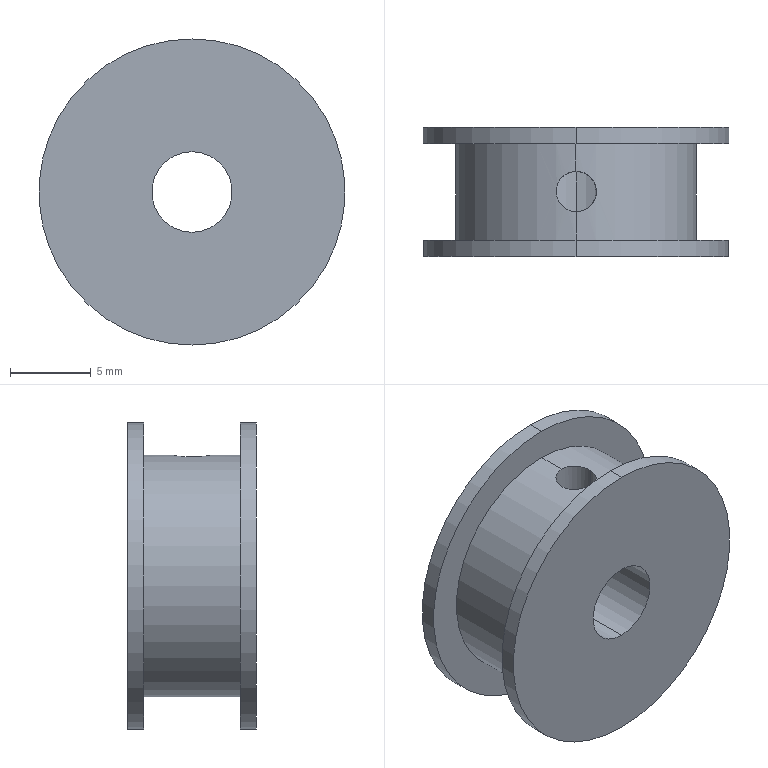Part | SolidWorks | features 3DProfileFeature 1, HoleWzd 1, Revolution 1 | 1 solid | 14 faces | box 19 x 8 x 19 mm | volume 1445 mm3 | cylinder 10 | plane 4 | commonest cylinder face diameters 19 x4 2.5 x2 5 x2 15 x2
STEP:
#1=CARTESIAN_POINT('',(-1.244,5.135,2.168));
#2=VERTEX_POINT('',#1);
#3=CARTESIAN_POINT('',(0.,3.885,2.5));
#4=VERTEX_POINT('',#3);
#5=CARTESIAN_POINT('',(-1.244,5.135,2.168));
#6=CARTESIAN_POINT('',(-1.244,5.053,2.168));
#7=CARTESIAN_POINT('',(-1.236,4.969,2.173));
#8=CARTESIAN_POINT('',(-1.203,4.808,2.191));
#9=CARTESIAN_POINT('',(-1.179,4.73,2.205));
#10=CARTESIAN_POINT('',(-1.085,4.503,2.253));
#11=CARTESIAN_POINT('',(-0.9937,4.368,2.297));
#12=CARTESIAN_POINT('',(-0.8237,4.197,2.361));
#13=CARTESIAN_POINT('',(-0.7622,4.146,2.382));
#14=CARTESIAN_POINT('',(-0.6291,4.056,2.421));
#15=CARTESIAN_POINT('',(-0.5566,4.016,2.438));
#16=CARTESIAN_POINT('',(-0.3321,3.921,2.483));
#17=CARTESIAN_POINT('',(-0.1673,3.886,2.5));
#18=CARTESIAN_POINT('',(0.,3.885,2.5));
#19=B_SPLINE_CURVE_WITH_KNOTS('',3,(#5,#6,#7,#8,#9,#10,#11,#12,#13,#14,#15,#16,#17,#18),.UNSPECIFIED.,.F.,.F.,(4,2,2,2,2,2,4),(0.005969,0.006216,0.006463,0.006957,0.007204,0.007451,0.007946),.UNSPECIFIED.);
#20=EDGE_CURVE('',#2,#4,#19,.T.);
#21=ORIENTED_EDGE('',*,*,#20,.F.);
#22=CARTESIAN_POINT('',(-1.231,5.135,7.398));
#23=VERTEX_POINT('',#22);
#24=CARTESIAN_POINT('',(-1.23,5.135,7.503));
#25=DIRECTION('',(0.002602,0.,1.));
#26=VECTOR('',#25,1000.);
#27=LINE('',#24,#26);
#28=EDGE_CURVE('',#2,#23,#27,.T.);
#29=ORIENTED_EDGE('',*,*,#28,.T.);
#30=CARTESIAN_POINT('',(0.,3.886,7.5));
#31=VERTEX_POINT('',#30);
#32=CARTESIAN_POINT('',(0.,3.886,7.5));
#33=CARTESIAN_POINT('',(-0.1639,3.888,7.5));
#34=CARTESIAN_POINT('',(-0.3241,3.923,7.494));
#35=CARTESIAN_POINT('',(-0.6224,4.051,7.476));
#36=CARTESIAN_POINT('',(-0.7586,4.144,7.462));
#37=CARTESIAN_POINT('',(-0.9848,4.374,7.436));
#38=CARTESIAN_POINT('',(-1.076,4.512,7.423));
#39=CARTESIAN_POINT('',(-1.198,4.811,7.404));
#40=CARTESIAN_POINT('',(-1.231,4.974,7.398));
#41=CARTESIAN_POINT('',(-1.231,5.135,7.398));
#42=B_SPLINE_CURVE_WITH_KNOTS('',3,(#32,#33,#34,#35,#36,#37,#38,#39,#40,#41),.UNSPECIFIED.,.F.,.F.,(4,2,2,2,4),(0.,0.0004846,0.0009692,0.001454,0.001938),.UNSPECIFIED.);
#43=EDGE_CURVE('',#31,#23,#42,.T.);
#44=ORIENTED_EDGE('',*,*,#43,.F.);
#45=CARTESIAN_POINT('',(1.269,5.135,7.392));
#46=VERTEX_POINT('',#45);
#47=CARTESIAN_POINT('',(1.269,5.135,7.392));
#48=CARTESIAN_POINT('',(1.269,4.969,7.392));
#49=CARTESIAN_POINT('',(1.236,4.805,7.398));
#50=CARTESIAN_POINT('',(1.108,4.5,7.418));
#51=CARTESIAN_POINT('',(1.014,4.36,7.432));
#52=CARTESIAN_POINT('',(0.7796,4.13,7.46));
#53=CARTESIAN_POINT('',(0.6382,4.037,7.474));
#54=CARTESIAN_POINT('',(0.3334,3.914,7.494));
#55=CARTESIAN_POINT('',(0.167,3.883,7.5));
#56=CARTESIAN_POINT('',(0.,3.886,7.5));
#57=B_SPLINE_CURVE_WITH_KNOTS('',3,(#47,#48,#49,#50,#51,#52,#53,#54,#55,#56),.UNSPECIFIED.,.F.,.F.,(4,2,2,2,4),(0.005853,0.006347,0.006841,0.007335,0.007829),.UNSPECIFIED.);
#58=EDGE_CURVE('',#46,#31,#57,.T.);
#59=ORIENTED_EDGE('',*,*,#58,.F.);
#60=CARTESIAN_POINT('',(1.256,5.135,2.162));
#61=VERTEX_POINT('',#60);
#62=CARTESIAN_POINT('',(1.27,5.135,7.497));
#63=DIRECTION('',(0.002602,0.,1.));
#64=VECTOR('',#63,1000.);
#65=LINE('',#62,#64);
#66=EDGE_CURVE('',#61,#46,#65,.T.);
#67=ORIENTED_EDGE('',*,*,#66,.F.);
#68=CARTESIAN_POINT('',(0.,3.885,2.5));
#69=CARTESIAN_POINT('',(0.08444,3.885,2.5));
#70=CARTESIAN_POINT('',(0.1673,3.893,2.496));
#71=CARTESIAN_POINT('',(0.3298,3.925,2.479));
#72=CARTESIAN_POINT('',(0.4104,3.95,2.467));
#73=CARTESIAN_POINT('',(0.638,4.044,2.422));
#74=CARTESIAN_POINT('',(0.7754,4.137,2.38));
#75=CARTESIAN_POINT('',(1.003,4.364,2.293));
#76=CARTESIAN_POINT('',(1.095,4.501,2.248));
#77=CARTESIAN_POINT('',(1.19,4.727,2.199));
#78=CARTESIAN_POINT('',(1.215,4.807,2.185));
#79=CARTESIAN_POINT('',(1.247,4.97,2.167));
#80=CARTESIAN_POINT('',(1.256,5.052,2.162));
#81=CARTESIAN_POINT('',(1.256,5.135,2.162));
#82=B_SPLINE_CURVE_WITH_KNOTS('',3,(#68,#69,#70,#71,#72,#73,#74,#75,#76,#77,#78,#79,#80,#81),.UNSPECIFIED.,.F.,.F.,(4,2,2,2,2,2,4),(0.,0.0002495,0.000499,0.0009979,0.001497,0.001746,0.001996),.UNSPECIFIED.);
#83=EDGE_CURVE('',#4,#61,#82,.T.);
#84=ORIENTED_EDGE('',*,*,#83,.F.);
#85=EDGE_LOOP('',(#21,#29,#44,#59,#67,#84));
#86=FACE_OUTER_BOUND('',#85,.T.);
#87=CARTESIAN_POINT('',(0.01951,5.135,7.5));
#88=DIRECTION('',(0.002602,0.,1.));
#89=DIRECTION('',(1.,0.,-0.002602));
#90=AXIS2_PLACEMENT_3D('',#87,#88,#89);
#91=CYLINDRICAL_SURFACE('',#90,1.25);
#92=ADVANCED_FACE('',(#86),#91,.F.);
#93=CARTESIAN_POINT('',(0.,1.117,-2.5));
#94=VERTEX_POINT('',#93);
#95=CARTESIAN_POINT('',(0.,1.117,2.5));
#96=VERTEX_POINT('',#95);
#97=CARTESIAN_POINT('',(0.,1.117,0.));
#98=DIRECTION('',(0.,1.,0.));
#99=DIRECTION('',(0.,0.,1.));
#100=AXIS2_PLACEMENT_3D('',#97,#98,#99);
#101=CIRCLE('',#100,2.5);
#102=EDGE_CURVE('',#94,#96,#101,.T.);
#103=ORIENTED_EDGE('',*,*,#102,.F.);
#104=CARTESIAN_POINT('',(0.,9.117,-2.5));
#105=VERTEX_POINT('',#104);
#106=CARTESIAN_POINT('',(0.,18.914,-2.5));
#107=DIRECTION('',(0.,1.,0.));
#108=VECTOR('',#107,1000.);
#109=LINE('',#106,#108);
#110=EDGE_CURVE('',#94,#105,#109,.T.);
#111=ORIENTED_EDGE('',*,*,#110,.T.);
#112=CARTESIAN_POINT('',(0.,9.117,2.5));
#113=VERTEX_POINT('',#112);
#114=CARTESIAN_POINT('',(0.,9.117,0.));
#115=DIRECTION('',(0.,1.,0.));
#116=DIRECTION('',(0.,0.,1.));
#117=AXIS2_PLACEMENT_3D('',#114,#115,#116);
#118=CIRCLE('',#117,2.5);
#119=EDGE_CURVE('',#105,#113,#118,.T.);
#120=ORIENTED_EDGE('',*,*,#119,.T.);
#121=CARTESIAN_POINT('',(0.,6.385,2.5));
#122=VERTEX_POINT('',#121);
#123=CARTESIAN_POINT('',(0.,18.914,2.5));
#124=DIRECTION('',(0.,1.,0.));
#125=VECTOR('',#124,1000.);
#126=LINE('',#123,#125);
#127=EDGE_CURVE('',#122,#113,#126,.T.);
#128=ORIENTED_EDGE('',*,*,#127,.F.);
#129=CARTESIAN_POINT('',(0.,6.385,2.5));
#130=CARTESIAN_POINT('',(-0.08271,6.385,2.5));
#131=CARTESIAN_POINT('',(-0.1668,6.376,2.496));
#132=CARTESIAN_POINT('',(-0.3281,6.343,2.48));
#133=CARTESIAN_POINT('',(-0.4065,6.318,2.468));
#134=CARTESIAN_POINT('',(-0.634,6.222,2.423));
#135=CARTESIAN_POINT('',(-0.7689,6.129,2.382));
#136=CARTESIAN_POINT('',(-0.9946,5.902,2.297));
#137=CARTESIAN_POINT('',(-1.086,5.765,2.253));
#138=CARTESIAN_POINT('',(-1.21,5.467,2.189));
#139=CARTESIAN_POINT('',(-1.244,5.3,2.168));
#140=CARTESIAN_POINT('',(-1.244,5.135,2.168));
#141=B_SPLINE_CURVE_WITH_KNOTS('',3,(#129,#130,#131,#132,#133,#134,#135,#136,#137,#138,#139,#140),.UNSPECIFIED.,.F.,.F.,(4,2,2,2,2,4),(0.003989,0.004237,0.004484,0.004979,0.005474,0.005969),.UNSPECIFIED.);
#142=EDGE_CURVE('',#122,#2,#141,.T.);
#143=ORIENTED_EDGE('',*,*,#142,.T.);
#144=ORIENTED_EDGE('',*,*,#20,.T.);
#145=CARTESIAN_POINT('',(0.,18.914,2.5));
#146=DIRECTION('',(0.,1.,0.));
#147=VECTOR('',#146,1000.);
#148=LINE('',#145,#147);
#149=EDGE_CURVE('',#96,#4,#148,.T.);
#150=ORIENTED_EDGE('',*,*,#149,.F.);
#151=EDGE_LOOP('',(#103,#111,#120,#128,#143,#144,#150));
#152=FACE_OUTER_BOUND('',#151,.T.);
#153=CARTESIAN_POINT('',(0.,18.914,0.));
#154=DIRECTION('',(0.,1.,0.));
#155=DIRECTION('',(0.,0.,1.));
#156=AXIS2_PLACEMENT_3D('',#153,#154,#155);
#157=CYLINDRICAL_SURFACE('',#156,2.5);
#158=ADVANCED_FACE('',(#152),#157,.F.);
#159=CARTESIAN_POINT('',(0.,1.117,9.5));
#160=VERTEX_POINT('',#159);
#161=CARTESIAN_POINT('',(0.,1.117,-9.5));
#162=VERTEX_POINT('',#161);
#163=CARTESIAN_POINT('',(0.,1.117,0.));
#164=DIRECTION('',(0.,1.,0.));
#165=DIRECTION('',(0.,0.,1.));
#166=AXIS2_PLACEMENT_3D('',#163,#164,#165);
#167=CIRCLE('',#166,9.5);
#168=EDGE_CURVE('',#160,#162,#167,.T.);
#169=ORIENTED_EDGE('',*,*,#168,.T.);
#170=CARTESIAN_POINT('',(0.,2.117,-9.5));
#171=VERTEX_POINT('',#170);
#172=CARTESIAN_POINT('',(0.,18.914,-9.5));
#173=DIRECTION('',(0.,1.,0.));
#174=VECTOR('',#173,1000.);
#175=LINE('',#172,#174);
#176=EDGE_CURVE('',#162,#171,#175,.T.);
#177=ORIENTED_EDGE('',*,*,#176,.T.);
#178=CARTESIAN_POINT('',(0.,2.117,9.5));
#179=VERTEX_POINT('',#178);
#180=CARTESIAN_POINT('',(0.,2.117,0.));
#181=DIRECTION('',(0.,1.,0.));
#182=DIRECTION('',(0.,0.,1.));
#183=AXIS2_PLACEMENT_3D('',#180,#181,#182);
#184=CIRCLE('',#183,9.5);
#185=EDGE_CURVE('',#179,#171,#184,.T.);
#186=ORIENTED_EDGE('',*,*,#185,.F.);
#187=CARTESIAN_POINT('',(0.,18.914,9.5));
#188=DIRECTION('',(0.,1.,0.));
#189=VECTOR('',#188,1000.);
#190=LINE('',#187,#189);
#191=EDGE_CURVE('',#160,#179,#190,.T.);
#192=ORIENTED_EDGE('',*,*,#191,.F.);
#193=EDGE_LOOP('',(#169,#177,#186,#192));
#194=FACE_OUTER_BOUND('',#193,.T.);
#195=CARTESIAN_POINT('',(0.,18.914,0.));
#196=DIRECTION('',(0.,1.,0.));
#197=DIRECTION('',(0.,0.,1.));
#198=AXIS2_PLACEMENT_3D('',#195,#196,#197);
#199=CYLINDRICAL_SURFACE('',#198,9.5);
#200=ADVANCED_FACE('',(#194),#199,.T.);
#201=CARTESIAN_POINT('',(0.,2.117,7.5));
#202=VERTEX_POINT('',#201);
#203=CARTESIAN_POINT('',(0.,2.117,-7.5));
#204=VERTEX_POINT('',#203);
#205=CARTESIAN_POINT('',(0.,2.117,0.));
#206=DIRECTION('',(0.,1.,0.));
#207=DIRECTION('',(0.,0.,1.));
#208=AXIS2_PLACEMENT_3D('',#205,#206,#207);
#209=CIRCLE('',#208,7.5);
#210=EDGE_CURVE('',#202,#204,#209,.T.);
#211=ORIENTED_EDGE('',*,*,#210,.T.);
#212=CARTESIAN_POINT('',(0.,8.117,-7.5));
#213=VERTEX_POINT('',#212);
#214=CARTESIAN_POINT('',(0.,18.914,-7.5));
#215=DIRECTION('',(0.,1.,0.));
#216=VECTOR('',#215,1000.);
#217=LINE('',#214,#216);
#218=EDGE_CURVE('',#204,#213,#217,.T.);
#219=ORIENTED_EDGE('',*,*,#218,.T.);
#220=CARTESIAN_POINT('',(0.,8.117,7.5));
#221=VERTEX_POINT('',#220);
#222=CARTESIAN_POINT('',(0.,8.117,0.));
#223=DIRECTION('',(0.,1.,0.));
#224=DIRECTION('',(0.,0.,1.));
#225=AXIS2_PLACEMENT_3D('',#222,#223,#224);
#226=CIRCLE('',#225,7.5);
#227=EDGE_CURVE('',#221,#213,#226,.T.);
#228=ORIENTED_EDGE('',*,*,#227,.F.);
#229=CARTESIAN_POINT('',(0.,6.385,7.5));
#230=VERTEX_POINT('',#229);
#231=CARTESIAN_POINT('',(0.,18.914,7.5));
#232=DIRECTION('',(0.,1.,0.));
#233=VECTOR('',#232,1000.);
#234=LINE('',#231,#233);
#235=EDGE_CURVE('',#230,#221,#234,.T.);
#236=ORIENTED_EDGE('',*,*,#235,.F.);
#237=CARTESIAN_POINT('',(0.,6.385,7.5));
#238=CARTESIAN_POINT('',(0.1653,6.388,7.5));
#239=CARTESIAN_POINT('',(0.3319,6.357,7.494));
#240=CARTESIAN_POINT('',(0.6374,6.234,7.474));
#241=CARTESIAN_POINT('',(0.779,6.142,7.46));
#242=CARTESIAN_POINT('',(1.013,5.911,7.432));
#243=CARTESIAN_POINT('',(1.108,5.772,7.418));
#244=CARTESIAN_POINT('',(1.236,5.467,7.398));
#245=CARTESIAN_POINT('',(1.269,5.303,7.392));
#246=CARTESIAN_POINT('',(1.269,5.135,7.392));
#247=B_SPLINE_CURVE_WITH_KNOTS('',3,(#237,#238,#239,#240,#241,#242,#243,#244,#245,#246),.UNSPECIFIED.,.F.,.F.,(4,2,2,2,4),(0.003876,0.00437,0.004865,0.005359,0.005853),.UNSPECIFIED.);
#248=EDGE_CURVE('',#230,#46,#247,.T.);
#249=ORIENTED_EDGE('',*,*,#248,.T.);
#250=ORIENTED_EDGE('',*,*,#58,.T.);
#251=CARTESIAN_POINT('',(0.,18.914,7.5));
#252=DIRECTION('',(0.,1.,0.));
#253=VECTOR('',#252,1000.);
#254=LINE('',#251,#253);
#255=EDGE_CURVE('',#202,#31,#254,.T.);
#256=ORIENTED_EDGE('',*,*,#255,.F.);
#257=EDGE_LOOP('',(#211,#219,#228,#236,#249,#250,#256));
#258=FACE_OUTER_BOUND('',#257,.T.);
#259=CARTESIAN_POINT('',(0.,18.914,0.));
#260=DIRECTION('',(0.,1.,0.));
#261=DIRECTION('',(0.,0.,1.));
#262=AXIS2_PLACEMENT_3D('',#259,#260,#261);
#263=CYLINDRICAL_SURFACE('',#262,7.5);
#264=ADVANCED_FACE('',(#258),#263,.T.);
#265=CARTESIAN_POINT('',(0.,8.117,9.5));
#266=VERTEX_POINT('',#265);
#267=CARTESIAN_POINT('',(0.,8.117,-9.5));
#268=VERTEX_POINT('',#267);
#269=CARTESIAN_POINT('',(0.,8.117,0.));
#270=DIRECTION('',(0.,1.,0.));
#271=DIRECTION('',(0.,0.,1.));
#272=AXIS2_PLACEMENT_3D('',#269,#270,#271);
#273=CIRCLE('',#272,9.5);
#274=EDGE_CURVE('',#266,#268,#273,.T.);
#275=ORIENTED_EDGE('',*,*,#274,.T.);
#276=CARTESIAN_POINT('',(0.,9.117,-9.5));
#277=VERTEX_POINT('',#276);
#278=CARTESIAN_POINT('',(0.,18.914,-9.5));
#279=DIRECTION('',(0.,1.,0.));
#280=VECTOR('',#279,1000.);
#281=LINE('',#278,#280);
#282=EDGE_CURVE('',#268,#277,#281,.T.);
#283=ORIENTED_EDGE('',*,*,#282,.T.);
#284=CARTESIAN_POINT('',(0.,9.117,9.5));
#285=VERTEX_POINT('',#284);
#286=CARTESIAN_POINT('',(0.,9.117,0.));
#287=DIRECTION('',(0.,1.,0.));
#288=DIRECTION('',(0.,0.,1.));
#289=AXIS2_PLACEMENT_3D('',#286,#287,#288);
#290=CIRCLE('',#289,9.5);
#291=EDGE_CURVE('',#285,#277,#290,.T.);
#292=ORIENTED_EDGE('',*,*,#291,.F.);
#293=CARTESIAN_POINT('',(0.,18.914,9.5));
#294=DIRECTION('',(0.,1.,0.));
#295=VECTOR('',#294,1000.);
#296=LINE('',#293,#295);
#297=EDGE_CURVE('',#266,#285,#296,.T.);
#298=ORIENTED_EDGE('',*,*,#297,.F.);
#299=EDGE_LOOP('',(#275,#283,#292,#298));
#300=FACE_OUTER_BOUND('',#299,.T.);
#301=CARTESIAN_POINT('',(0.,18.914,0.));
#302=DIRECTION('',(0.,1.,0.));
#303=DIRECTION('',(0.,0.,1.));
#304=AXIS2_PLACEMENT_3D('',#301,#302,#303);
#305=CYLINDRICAL_SURFACE('',#304,9.5);
#306=ADVANCED_FACE('',(#300),#305,.T.);
#307=ORIENTED_EDGE('',*,*,#282,.F.);
#308=CARTESIAN_POINT('',(0.,8.117,0.));
#309=DIRECTION('',(0.,1.,0.));
#310=DIRECTION('',(0.,0.,1.));
#311=AXIS2_PLACEMENT_3D('',#308,#309,#310);
#312=CIRCLE('',#311,9.5);
#313=EDGE_CURVE('',#268,#266,#312,.T.);
#314=ORIENTED_EDGE('',*,*,#313,.T.);
#315=ORIENTED_EDGE('',*,*,#297,.T.);
#316=CARTESIAN_POINT('',(0.,9.117,0.));
#317=DIRECTION('',(0.,1.,0.));
#318=DIRECTION('',(0.,0.,1.));
#319=AXIS2_PLACEMENT_3D('',#316,#317,#318);
#320=CIRCLE('',#319,9.5);
#321=EDGE_CURVE('',#277,#285,#320,.T.);
#322=ORIENTED_EDGE('',*,*,#321,.F.);
#323=EDGE_LOOP('',(#307,#314,#315,#322));
#324=FACE_OUTER_BOUND('',#323,.T.);
#325=CARTESIAN_POINT('',(0.,18.914,0.));
#326=DIRECTION('',(0.,1.,0.));
#327=DIRECTION('',(0.,0.,1.));
#328=AXIS2_PLACEMENT_3D('',#325,#326,#327);
#329=CYLINDRICAL_SURFACE('',#328,9.5);
#330=ADVANCED_FACE('',(#324),#329,.T.);
#331=ORIENTED_EDGE('',*,*,#274,.F.);
#332=ORIENTED_EDGE('',*,*,#313,.F.);
#333=EDGE_LOOP('',(#331,#332));
#334=FACE_OUTER_BOUND('',#333,.T.);
#335=ORIENTED_EDGE('',*,*,#227,.T.);
#336=CARTESIAN_POINT('',(0.,8.117,0.));
#337=DIRECTION('',(0.,1.,0.));
#338=DIRECTION('',(0.,0.,1.));
#339=AXIS2_PLACEMENT_3D('',#336,#337,#338);
#340=CIRCLE('',#339,7.5);
#341=EDGE_CURVE('',#213,#221,#340,.T.);
#342=ORIENTED_EDGE('',*,*,#341,.T.);
#343=EDGE_LOOP('',(#335,#342));
#344=FACE_BOUND('',#343,.T.);
#345=CARTESIAN_POINT('',(9.5,8.117,0.));
#346=DIRECTION('',(0.,1.,0.));
#347=DIRECTION('',(0.,0.,1.));
#348=AXIS2_PLACEMENT_3D('',#345,#346,#347);
#349=PLANE('',#348);
#350=ADVANCED_FACE('',(#334,#344),#349,.F.);
#351=ORIENTED_EDGE('',*,*,#218,.F.);
#352=CARTESIAN_POINT('',(0.,2.117,0.));
#353=DIRECTION('',(0.,1.,0.));
#354=DIRECTION('',(0.,0.,1.));
#355=AXIS2_PLACEMENT_3D('',#352,#353,#354);
#356=CIRCLE('',#355,7.5);
#357=EDGE_CURVE('',#204,#202,#356,.T.);
#358=ORIENTED_EDGE('',*,*,#357,.T.);
#359=ORIENTED_EDGE('',*,*,#255,.T.);
#360=ORIENTED_EDGE('',*,*,#43,.T.);
#361=CARTESIAN_POINT('',(-1.231,5.135,7.398));
#362=CARTESIAN_POINT('',(-1.231,5.297,7.398));
#363=CARTESIAN_POINT('',(-1.199,5.46,7.404));
#364=CARTESIAN_POINT('',(-1.076,5.759,7.423));
#365=CARTESIAN_POINT('',(-0.9857,5.896,7.436));
#366=CARTESIAN_POINT('',(-0.7572,6.128,7.463));
#367=CARTESIAN_POINT('',(-0.6222,6.22,7.476));
#368=CARTESIAN_POINT('',(-0.398,6.316,7.49));
#369=CARTESIAN_POINT('',(-0.3211,6.341,7.494));
#370=CARTESIAN_POINT('',(-0.163,6.375,7.499));
#371=CARTESIAN_POINT('',(-0.08099,6.384,7.5));
#372=CARTESIAN_POINT('',(0.,6.385,7.5));
#373=B_SPLINE_CURVE_WITH_KNOTS('',3,(#361,#362,#363,#364,#365,#366,#367,#368,#369,#370,#371,#372),.UNSPECIFIED.,.F.,.F.,(4,2,2,2,2,4),(0.001938,0.002423,0.002907,0.003392,0.003634,0.003876),.UNSPECIFIED.);
#374=EDGE_CURVE('',#23,#230,#373,.T.);
#375=ORIENTED_EDGE('',*,*,#374,.T.);
#376=ORIENTED_EDGE('',*,*,#235,.T.);
#377=ORIENTED_EDGE('',*,*,#341,.F.);
#378=EDGE_LOOP('',(#351,#358,#359,#360,#375,#376,#377));
#379=FACE_OUTER_BOUND('',#378,.T.);
#380=CARTESIAN_POINT('',(0.,18.914,0.));
#381=DIRECTION('',(0.,1.,0.));
#382=DIRECTION('',(0.,0.,1.));
#383=AXIS2_PLACEMENT_3D('',#380,#381,#382);
#384=CYLINDRICAL_SURFACE('',#383,7.5);
#385=ADVANCED_FACE('',(#379),#384,.T.);
#386=ORIENTED_EDGE('',*,*,#210,.F.);
#387=ORIENTED_EDGE('',*,*,#357,.F.);
#388=EDGE_LOOP('',(#386,#387));
#389=FACE_BOUND('',#388,.T.);
#390=ORIENTED_EDGE('',*,*,#185,.T.);
#391=CARTESIAN_POINT('',(0.,2.117,0.));
#392=DIRECTION('',(0.,1.,0.));
#393=DIRECTION('',(0.,0.,1.));
#394=AXIS2_PLACEMENT_3D('',#391,#392,#393);
#395=CIRCLE('',#394,9.5);
#396=EDGE_CURVE('',#171,#179,#395,.T.);
#397=ORIENTED_EDGE('',*,*,#396,.T.);
#398=EDGE_LOOP('',(#390,#397));
#399=FACE_OUTER_BOUND('',#398,.T.);
#400=CARTESIAN_POINT('',(7.5,2.117,0.));
#401=DIRECTION('',(0.,-1.,0.));
#402=DIRECTION('',(0.,0.,-1.));
#403=AXIS2_PLACEMENT_3D('',#400,#401,#402);
#404=PLANE('',#403);
#405=ADVANCED_FACE('',(#389,#399),#404,.F.);
#406=ORIENTED_EDGE('',*,*,#176,.F.);
#407=CARTESIAN_POINT('',(0.,1.117,0.));
#408=DIRECTION('',(0.,1.,0.));
#409=DIRECTION('',(0.,0.,1.));
#410=AXIS2_PLACEMENT_3D('',#407,#408,#409);
#411=CIRCLE('',#410,9.5);
#412=EDGE_CURVE('',#162,#160,#411,.T.);
#413=ORIENTED_EDGE('',*,*,#412,.T.);
#414=ORIENTED_EDGE('',*,*,#191,.T.);
#415=ORIENTED_EDGE('',*,*,#396,.F.);
#416=EDGE_LOOP('',(#406,#413,#414,#415));
#417=FACE_OUTER_BOUND('',#416,.T.);
#418=CARTESIAN_POINT('',(0.,18.914,0.));
#419=DIRECTION('',(0.,1.,0.));
#420=DIRECTION('',(0.,0.,1.));
#421=AXIS2_PLACEMENT_3D('',#418,#419,#420);
#422=CYLINDRICAL_SURFACE('',#421,9.5);
#423=ADVANCED_FACE('',(#417),#422,.T.);
#424=ORIENTED_EDGE('',*,*,#168,.F.);
#425=ORIENTED_EDGE('',*,*,#412,.F.);
#426=EDGE_LOOP('',(#424,#425));
#427=FACE_OUTER_BOUND('',#426,.T.);
#428=CARTESIAN_POINT('',(0.,1.117,0.));
#429=DIRECTION('',(0.,1.,0.));
#430=DIRECTION('',(0.,0.,1.));
#431=AXIS2_PLACEMENT_3D('',#428,#429,#430);
#432=CIRCLE('',#431,2.5);
#433=EDGE_CURVE('',#96,#94,#432,.T.);
#434=ORIENTED_EDGE('',*,*,#433,.T.);
#435=ORIENTED_EDGE('',*,*,#102,.T.);
#436=EDGE_LOOP('',(#434,#435));
#437=FACE_BOUND('',#436,.T.);
#438=CARTESIAN_POINT('',(9.5,1.117,0.));
#439=DIRECTION('',(0.,1.,0.));
#440=DIRECTION('',(0.,0.,1.));
#441=AXIS2_PLACEMENT_3D('',#438,#439,#440);
#442=PLANE('',#441);
#443=ADVANCED_FACE('',(#427,#437),#442,.F.);
#444=ORIENTED_EDGE('',*,*,#110,.F.);
#445=ORIENTED_EDGE('',*,*,#433,.F.);
#446=ORIENTED_EDGE('',*,*,#149,.T.);
#447=ORIENTED_EDGE('',*,*,#83,.T.);
#448=CARTESIAN_POINT('',(1.256,5.135,2.162));
#449=CARTESIAN_POINT('',(1.256,5.302,2.162));
#450=CARTESIAN_POINT('',(1.221,5.469,2.183));
#451=CARTESIAN_POINT('',(1.094,5.772,2.249));
#452=CARTESIAN_POINT('',(1.001,5.909,2.294));
#453=CARTESIAN_POINT('',(0.7735,6.135,2.38));
#454=CARTESIAN_POINT('',(0.6356,6.228,2.423));
#455=CARTESIAN_POINT('',(0.3342,6.353,2.482));
#456=CARTESIAN_POINT('',(0.1666,6.386,2.5));
#457=CARTESIAN_POINT('',(0.,6.385,2.5));
#458=B_SPLINE_CURVE_WITH_KNOTS('',3,(#448,#449,#450,#451,#452,#453,#454,#455,#456,#457),.UNSPECIFIED.,.F.,.F.,(4,2,2,2,4),(0.001996,0.002494,0.002993,0.003491,0.003989),.UNSPECIFIED.);
#459=EDGE_CURVE('',#61,#122,#458,.T.);
#460=ORIENTED_EDGE('',*,*,#459,.T.);
#461=ORIENTED_EDGE('',*,*,#127,.T.);
#462=CARTESIAN_POINT('',(0.,9.117,0.));
#463=DIRECTION('',(0.,1.,0.));
#464=DIRECTION('',(0.,0.,1.));
#465=AXIS2_PLACEMENT_3D('',#462,#463,#464);
#466=CIRCLE('',#465,2.5);
#467=EDGE_CURVE('',#113,#105,#466,.T.);
#468=ORIENTED_EDGE('',*,*,#467,.T.);
#469=EDGE_LOOP('',(#444,#445,#446,#447,#460,#461,#468));
#470=FACE_OUTER_BOUND('',#469,.T.);
#471=CARTESIAN_POINT('',(0.,18.914,0.));
#472=DIRECTION('',(0.,1.,0.));
#473=DIRECTION('',(0.,0.,1.));
#474=AXIS2_PLACEMENT_3D('',#471,#472,#473);
#475=CYLINDRICAL_SURFACE('',#474,2.5);
#476=ADVANCED_FACE('',(#470),#475,.F.);
#477=ORIENTED_EDGE('',*,*,#467,.F.);
#478=ORIENTED_EDGE('',*,*,#119,.F.);
#479=EDGE_LOOP('',(#477,#478));
#480=FACE_BOUND('',#479,.T.);
#481=ORIENTED_EDGE('',*,*,#291,.T.);
#482=ORIENTED_EDGE('',*,*,#321,.T.);
#483=EDGE_LOOP('',(#481,#482));
#484=FACE_OUTER_BOUND('',#483,.T.);
#485=CARTESIAN_POINT('',(9.5,9.117,0.));
#486=DIRECTION('',(0.,-1.,0.));
#487=DIRECTION('',(0.,0.,-1.));
#488=AXIS2_PLACEMENT_3D('',#485,#486,#487);
#489=PLANE('',#488);
#490=ADVANCED_FACE('',(#480,#484),#489,.F.);
#491=ORIENTED_EDGE('',*,*,#28,.F.);
#492=ORIENTED_EDGE('',*,*,#142,.F.);
#493=ORIENTED_EDGE('',*,*,#459,.F.);
#494=ORIENTED_EDGE('',*,*,#66,.T.);
#495=ORIENTED_EDGE('',*,*,#248,.F.);
#496=ORIENTED_EDGE('',*,*,#374,.F.);
#497=EDGE_LOOP('',(#491,#492,#493,#494,#495,#496));
#498=FACE_OUTER_BOUND('',#497,.T.);
#499=CARTESIAN_POINT('',(0.01951,5.135,7.5));
#500=DIRECTION('',(0.002602,0.,1.));
#501=DIRECTION('',(1.,0.,-0.002602));
#502=AXIS2_PLACEMENT_3D('',#499,#500,#501);
#503=CYLINDRICAL_SURFACE('',#502,1.25);
#504=ADVANCED_FACE('',(#498),#503,.F.);
#505=CLOSED_SHELL('',(#92,#158,#200,#264,#306,#330,#350,#385,#405,#423,#443,#476,#490,#504));
#506=MANIFOLD_SOLID_BREP('',#505);
#507=CARTESIAN_POINT('',(0.,0.,0.));
#508=DIRECTION('',(0.,0.,1.));
#509=DIRECTION('',(1.,0.,0.));
#510=AXIS2_PLACEMENT_3D('',#507,#508,#509);
#511=(LENGTH_UNIT()NAMED_UNIT(*)SI_UNIT(.MILLI.,.METRE.));
#512=UNCERTAINTY_MEASURE_WITH_UNIT(LENGTH_MEASURE(0.00001),#511,'','');
#513=(NAMED_UNIT(*)PLANE_ANGLE_UNIT()SI_UNIT($,.RADIAN.));
#514=(NAMED_UNIT(*)SI_UNIT($,.STERADIAN.)SOLID_ANGLE_UNIT());
#515=(GEOMETRIC_REPRESENTATION_CONTEXT(3)GLOBAL_UNCERTAINTY_ASSIGNED_CONTEXT((#512))GLOBAL_UNIT_ASSIGNED_CONTEXT((#511,#513,#514))REPRESENTATION_CONTEXT('',''));
#516=ADVANCED_BREP_SHAPE_REPRESENTATION('',(#506,#510),#515);